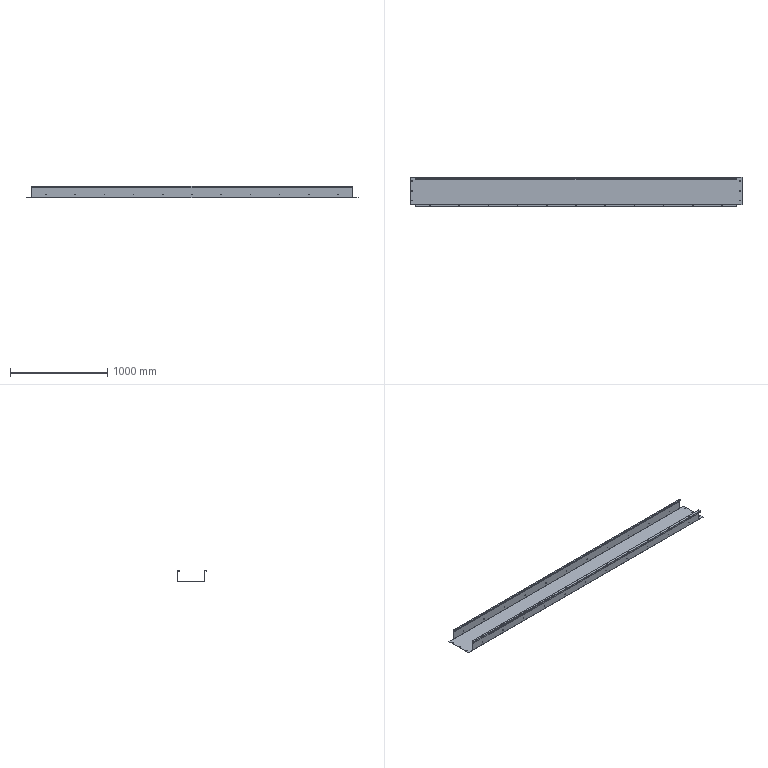Part | STEP file | TS-S82 | 1 solid | 192 faces | box 3411 x 303 x 122 mm | volume 3873447 mm3 | cylinder 112 | plane 80 | commonest cylinder face diameters 5.4 x66 8 x22 7 x12 0.4 x6 4.4 x6